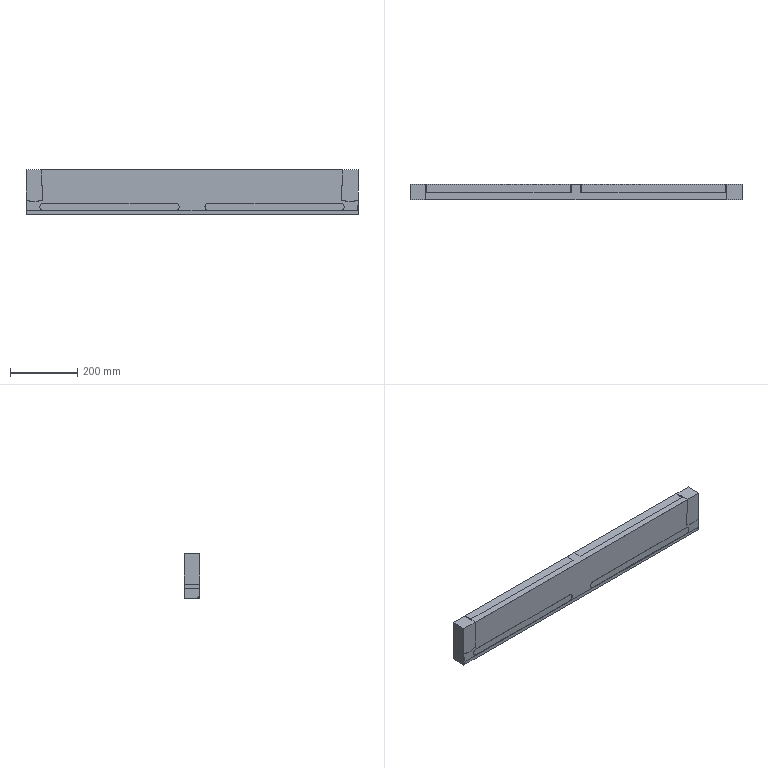NC program | NX | posted with a generic post | part box 987 x 45 x 132.5 mm
Whole program:
N10 G17 G21 G94 G90
(ZLEVEL_PROFILE_COPY_2 , TOOL : D63)
N12 T01 M6
N14 G54
N16 G17 G0 G90 X542.392 Y-19.114 B0. C0. S6500 M3
N18 G43 Z30. H1
N20 Z5.625
N22 G94 G1 X537.561 Y-10.747 F2000.
N24 G3 X532.106 Y-7.597 R6.3
N26 G1 X500.977
N28 X498.032 Y-7.6
N30 X-491.979
N32 X-532.106 Y-7.597
N34 G3 X-537.562 Y-10.746 R6.3
N36 G1 X-542.393 Y-19.113
N38 G0 Z3.75
N40 G1 X-537.562 Y-10.746
N42 G2 X-532.106 Y-7.597 R6.3
N44 G1 X-491.979 Y-7.6
N46 X498.032
N48 X500.977 Y-7.597
N50 X532.106
N52 G2 X537.561 Y-10.747 R6.3
N54 G1 X542.392 Y-19.114
N56 G0 Z1.875
N58 G1 X537.561 Y-10.747
N60 G3 X532.106 Y-7.597 R6.3
N62 G1 X500.977
N64 X498.032 Y-7.6
N66 X-491.979
N68 X-532.106 Y-7.597
N70 G3 X-537.562 Y-10.747 R6.3
N72 G1 X-542.393 Y-19.113
N74 G0 Z0.
N76 G1 X-537.562 Y-10.747
N78 G2 X-532.106 Y-7.597 R6.3
N80 G1 X-491.979 Y-7.6
N82 X498.032
N84 X500.977 Y-7.597
N86 X532.106
N88 G2 X537.561 Y-10.747 R6.3
N90 G1 X542.392 Y-19.114
N92 G0 Z30.
(ZLEVEL_PROFILE , TOOL : D63)
N94 X489.437 Y67.209
N96 Z-1.968
N98 G1 X481.147 Y62.423
N100 G3 X477.997 Y56.967 R6.3
N102 G1 Y24.501
N104 X478. Y22.551
N106 Y-16.867
N108 X477.997 Y-56.967
N110 G3 X481.147 Y-62.423 R6.3
N112 G1 X489.437 Y-67.211
N114 G0 Z-3.936
N116 G1 X481.147 Y-62.423
N118 G2 X477.997 Y-56.967 R6.3
N120 G1 X478. Y-16.867
N122 Y22.551
N124 X477.997 Y24.501
N126 Y56.967
N128 G2 X481.147 Y62.423 R6.3
N130 G1 X489.437 Y67.209
N132 G0 X489.438 Z-5.904
N134 G1 X481.147 Y62.423
N136 G3 X477.997 Y56.967 R6.3
N138 G1 Y24.501
N140 X478. Y22.551
N142 Y-16.867
N144 X477.997 Y-56.967
N146 G3 X481.147 Y-62.423 R6.3
N148 G1 X489.437 Y-67.21
N150 G0 Z-7.872
N152 G1 X481.147 Y-62.423
N154 G2 X477.997 Y-56.967 R6.3
N156 G1 X478. Y-16.867
N158 Y22.551
N160 X477.997 Y24.501
N162 Y56.967
N164 G2 X481.147 Y62.423 R6.3
N166 G1 X489.438 Y67.209
N168 G0 Z-9.84
N170 G1 X481.147 Y62.423
N172 G3 X477.997 Y56.967 R6.3
N174 G1 Y24.501
N176 X478. Y22.551
N178 Y-16.867
N180 X477.997 Y-56.967
N182 G3 X481.147 Y-62.423 R6.3
N184 G1 X489.437 Y-67.21
N186 G0 X489.438 Z-11.809
N188 G1 X481.147 Y-62.423
N190 G2 X477.997 Y-56.967 R6.3
N192 G1 X478. Y-16.867
N194 Y22.551
N196 X477.997 Y24.501
N198 Y56.967
N200 G2 X481.147 Y62.423 R6.3
N202 G1 X489.438 Y67.209
N204 G0 Y67.21 Z-13.777
N206 G1 X481.147 Y62.423
N208 G3 X477.997 Y56.967 R6.3
N210 G1 Y24.501
N212 X478. Y22.551
N214 Y-16.867
N216 X477.997 Y-56.967
N218 G3 X481.147 Y-62.423 R6.3
N220 G1 X489.44 Y-67.212
N222 G0 Y-67.211 Z-15.745
N224 G1 X481.147 Y-62.423
N226 G2 X477.998 Y-56.967 R6.3
N228 G1 X478. Y-16.867
N230 Y22.551
N232 X477.998 Y24.501
N234 Y56.967
N236 G2 X481.148 Y62.423 R6.3
N238 G1 X489.438 Y67.21
N240 G0 Z-17.713
N242 G1 X481.148 Y62.423
N244 G3 X477.998 Y56.967 R6.3
N246 G1 Y24.501
N248 X478. Y22.551
N250 Y-16.867
N252 X477.998 Y-56.967
N254 G3 X481.147 Y-62.423 R6.3
N256 G1 X489.438 Y-67.21
N258 G0 Z-19.681
N260 G1 X481.147 Y-62.423
N262 G2 X477.998 Y-56.967 R6.3
N264 G1 X478. Y-16.867
N266 Y22.551
N268 X477.998 Y24.501
N270 Y56.967
N272 G2 X481.148 Y62.423 R6.3
N274 G1 X489.438 Y67.21
N276 G0 Z-21.649
N278 G1 X481.148 Y62.423
N280 G3 X477.998 Y56.967 R6.3
N282 G1 Y24.501
N284 X478. Y22.551
N286 Y-16.867
N288 X477.998 Y-56.967
N290 G3 X481.147 Y-62.423 R6.3
N292 G1 X489.438 Y-67.21
N294 G0 Z-23.617
N296 G1 X481.148 Y-62.423
N298 G2 X477.998 Y-56.967 R6.3
N300 G1 X478. Y-16.867
N302 Y22.551
N304 X477.998 Y24.501
N306 Y56.967
N308 G2 X481.148 Y62.423 R6.3
N310 G1 X489.438 Y67.21
N312 G0 Z-25.585
N314 G1 X481.148 Y62.423
N316 G3 X477.998 Y56.967 R6.3
N318 G1 Y24.501
N320 X478. Y22.551
N322 Y-16.867
N324 X477.998 Y-56.967
N326 G3 X481.148 Y-62.423 R6.3
N328 G1 X489.438 Y-67.21
N330 G0 Z-27.553
N332 G1 X481.148 Y-62.423
N334 G2 X477.998 Y-56.967 R6.3
N336 G1 X478. Y-16.867
N338 Y22.551
N340 X477.998 Y24.501
N342 Y56.967
N344 G2 X481.148 Y62.423 R6.3
N346 G1 X489.438 Y67.21
N348 G0 Z-29.521
N350 G1 X481.148 Y62.423
N352 G3 X477.998 Y56.967 R6.3
N354 G1 X478. Y22.551
N356 Y-16.867
N358 X477.998 Y-56.967
N360 G3 X481.148 Y-62.423 R6.3
N362 G1 X489.438 Y-67.21
N364 G0 Z-31.489
N366 G1 X481.148 Y-62.423
N368 G2 X477.998 Y-56.967 R6.3
N370 G1 X478. Y-16.867
N372 Y22.551
N374 X477.998 Y56.967
N376 G2 X481.148 Y62.423 R6.3
N378 G1 X489.438 Y67.21
N380 G0 X489.44 Y67.211 Z-33.457
N382 G1 X481.148 Y62.423
N384 G3 X477.998 Y56.967 R6.3
N386 G1 X478. Y22.551
N388 Y-16.867
N390 X477.998 Y-56.967
N392 G3 X481.148 Y-62.423 R6.3
N394 G1 X489.44 Y-67.211
N396 G0 Z-35.426
N398 G1 X481.148 Y-62.423
N400 G2 X477.998 Y-56.967 R6.3
N402 G1 X478. Y-16.867
N404 Y22.551
N406 X477.998 Y56.967
N408 G2 X481.148 Y62.423 R6.3
N410 G1 X489.44 Y67.211
N412 G0 X489.441 Z-37.394
N414 G1 X481.148 Y62.423
N416 G3 X477.998 Y56.967 R6.3
N418 G1 X478. Y22.551
N420 Y-16.867
N422 X477.998 Y-56.967
N424 G3 X481.148 Y-62.423 R6.3
N426 G1 X489.441 Y-67.211
N428 G0 Z-39.362
N430 G1 X481.148 Y-62.423
N432 G2 X477.998 Y-56.967 R6.3
N434 G1 X478. Y-16.867
N436 Y22.551
N438 X477.998 Y56.967
N440 G2 X481.148 Y62.423 R6.3
N442 G1 X489.441 Y67.211
N444 G0 Z-41.33
N446 G1 X481.148 Y62.423
N448 G3 X477.998 Y56.967 R6.3
N450 G1 X478. Y22.551
N452 Y-16.867
N454 X477.998 Y-56.967
N456 G3 X481.148 Y-62.423 R6.3
N458 G1 X489.441 Y-67.211
N460 G0 Z-43.298
N462 G1 X481.148 Y-62.423
N464 G2 X477.999 Y-56.967 R6.3
N466 G1 X478. Y-16.867
N468 Y22.551
N470 X477.999 Y56.967
N472 G2 X481.148 Y62.423 R6.3
N474 G1 X489.441 Y67.211
N476 G0 Z-45.266
N478 G1 X481.148 Y62.423
N480 G3 X477.999 Y56.967 R6.3
N482 G1 X478. Y22.551
N484 Y-16.867
N486 X477.999 Y-56.967
N488 G3 X481.148 Y-62.423 R6.3
N490 G1 X489.441 Y-67.211
N492 G0 Z-47.234
N494 G1 X481.149 Y-62.423
N496 G2 X477.999 Y-56.967 R6.3
N498 G1 X478. Y-16.867
N500 Y22.551
N502 X477.999 Y56.967
N504 G2 X481.148 Y62.423 R6.3
N506 G1 X489.441 Y67.211
N508 G0 Z-49.202
N510 G1 X481.149 Y62.423
N512 G3 X477.999 Y56.967 R6.3
N514 G1 X478. Y22.551
N516 Y-16.867
N518 X477.999 Y-56.967
N520 G3 X481.149 Y-62.423 R6.3
N522 G1 X489.441 Y-67.211
N524 G0 Z-51.17
N526 G1 X481.149 Y-62.423
N528 G2 X477.999 Y-56.967 R6.3
N530 G1 X478. Y-16.867
N532 Y22.551
N534 X477.999 Y56.967
N536 G2 X481.149 Y62.423 R6.3
N538 G1 X489.441 Y67.211
N540 G0 Z-53.138
N542 G1 X481.149 Y62.423
N544 G3 X477.999 Y56.967 R6.3
N546 G1 X478. Y22.551
N548 Y-16.867
N550 X477.999 Y-56.967
N552 G3 X481.149 Y-62.423 R6.3
N554 G1 X489.441 Y-67.211
N556 G0 Z-55.106
N558 G1 X481.149 Y-62.423
N560 G2 X477.999 Y-56.967 R6.3
N562 G1 X478. Y-16.867
N564 Y22.551
N566 X477.999 Y56.967
N568 G2 X481.149 Y62.423 R6.3
N570 G1 X489.441 Y67.211
N572 G0 Z-57.074
N574 G1 X481.149 Y62.423
N576 G3 X477.999 Y56.967 R6.3
N578 G1 X478. Y22.551
N580 Y-16.867
N582 X477.999 Y-56.967
N584 G3 X481.149 Y-62.423 R6.3
N586 G1 X489.441 Y-67.211
N588 G0 Z-59.043
N590 G1 X481.149 Y-62.423
N592 G2 X477.999 Y-56.967 R6.3
N594 G1 X478. Y-16.867
N596 Y22.551
N598 X477.999 Y56.967
N600 G2 X481.149 Y62.423 R6.3
N602 G1 X489.441 Y67.211
N604 G0 Z-61.011
N606 G1 X481.149 Y62.423
N608 G3 X477.999 Y56.967 R6.3
N610 G1 X478. Y22.551
N612 Y-16.867
N614 X477.999 Y-56.967
N616 G3 X481.149 Y-62.423 R6.3
N618 G1 X489.441 Y-67.211
N620 G0 Z-62.979
N622 G1 X481.149 Y-62.423
N624 G2 X477.999 Y-56.967 R6.3
N626 G1 X478. Y-16.867
N628 Y22.551
N630 X477.999 Y56.967
N632 G2 X481.149 Y62.423 R6.3
N634 G1 X489.441 Y67.211
N636 G0 X489.442 Z-64.947
N638 G1 X481.149 Y62.423
N640 G3 X477.999 Y56.967 R6.3
N642 G1 X478. Y22.551
N644 Y-16.867
N646 X477.999 Y-56.967
N648 G3 X481.149 Y-62.423 R6.3
N650 G1 X489.442 Y-67.211
N652 G0 Z-66.915
N654 G1 X481.149 Y-62.423
N656 G2 X477.999 Y-56.967 R6.3
N658 G1 X478. Y-16.867
N660 Y22.551
N662 X477.999 Y56.967
N664 G2 X481.149 Y62.423 R6.3
N666 G1 X489.442 Y67.211
N668 G0 Z-68.883
N670 G1 X481.149 Y62.423
N672 G3 X477.999 Y56.967 R6.3
N674 G1 X478. Y22.551
N676 Y-16.867
N678 X477.999 Y-56.967
N680 G3 X481.149 Y-62.423 R6.3
N682 G1 X489.442 Y-67.211
N684 G0 Z-70.851
N686 G1 X481.15 Y-62.423
N688 G2 X478. Y-56.967 R6.3
N690 G1 Y-16.867
N692 Y22.551
N694 Y56.967
N696 G2 X481.149 Y62.423 R6.3
N698 G1 X489.442 Y67.211
N700 G0 Z-72.819
N702 G1 X481.15 Y62.423
N704 G3 X478. Y56.967 R6.3
N706 G1 Y22.551
N708 Y-16.867
N710 Y-56.967
N712 G3 X481.15 Y-62.423 R6.3
N714 G1 X489.442 Y-67.211
N716 G0 Z-74.787
N718 G1 X481.15 Y-62.423
N720 G2 X478. Y-56.967 R6.3
N722 G1 Y-16.867
N724 Y22.551
N726 Y56.967
N728 G2 X481.15 Y62.423 R6.3
N730 G1 X489.442 Y67.211
N732 G0 Z-76.755
N734 G1 X481.15 Y62.423
N736 G3 X478. Y56.967 R6.3
N738 G1 Y22.551
N740 Y-16.867
N742 Y-56.967
N744 G3 X481.15 Y-62.423 R6.3
N746 G1 X489.442 Y-67.211
N748 G0 Z-78.723
N750 G1 X481.15 Y-62.423
N752 G2 X478. Y-56.967 R6.3
N754 G1 Y-16.867
N756 Y22.551
N758 Y56.967
N760 G2 X481.15 Y62.423 R6.3
N762 G1 X489.442 Y67.211
N764 G0 Z-80.691
N766 G1 X481.15 Y62.423
N768 G3 X478. Y56.967 R6.3
N770 G1 Y22.551
N772 Y-16.867
N774 Y-56.967
N776 G3 X481.15 Y-62.423 R6.3
N778 G1 X489.442 Y-67.211
N780 G0 Z-82.66
N782 G1 X481.15 Y-62.423
N784 G2 X478. Y-56.967 R6.3
N786 G1 Y-16.867
N788 Y22.463
N790 Y56.967
N792 G2 X481.15 Y62.423 R6.3
N794 G1 X489.442 Y67.211
N796 G0 Z-84.628
N798 G1 X481.15 Y62.423
N800 G3 X478. Y56.967 R6.3
N802 G1 Y22.463
N804 Y-16.867
N806 Y-56.967
N808 G3 X481.15 Y-62.423 R6.3
N810 G1 X489.442 Y-67.211
N812 G0 Z-86.596
N814 G1 X481.15 Y-62.423
N816 G2 X478. Y-56.967 R6.3
N818 G1 Y-16.867
N820 Y22.463
N822 Y56.967
N824 G2 X481.15 Y62.423 R6.3
N826 G1 X489.442 Y67.211
N828 G0 Z-88.564
N830 G1 X481.15 Y62.423
N832 G3 X478. Y56.967 R6.3
N834 G1 Y22.463
N836 Y-16.867
N838 Y-56.967
N840 G3 X481.15 Y-62.423 R6.3
N842 G1 X489.442 Y-67.211
N844 G0 Z-90.532
N846 G1 X481.15 Y-62.423
N848 G2 X478. Y-56.967 R6.3
N850 G1 Y-16.867
N852 Y22.463
N854 Y56.967
N856 G2 X481.15 Y62.423 R6.3
N858 G1 X489.442 Y67.211
N860 G0 Z-92.5
N862 G1 X481.15 Y62.423
N864 G3 X478. Y56.967 R6.3
N866 G1 Y22.463
N868 Y-16.867
N870 Y-56.967
N872 G3 X481.15 Y-62.423 R6.3
N874 G1 X489.442 Y-67.211
N876 G0 Z30.
N878 X-489.437
N880 Z-1.968
N882 G1 X-481.147 Y-62.423
N884 G3 X-477.997 Y-56.967 R6.3
N886 G1 X-478. Y-16.897
N888 Y22.5
N890 X-477.997 Y56.967
N892 G3 X-481.147 Y62.423 R6.3
N894 G1 X-489.437 Y67.211
N896 G0 X-489.435 Y67.218 Z-3.936
N898 G1 X-481.144 Y62.425
N900 G2 X-477.997 Y56.967 R6.3
N902 G1 X-477.999 Y53.105
N904 X-478. Y22.5
N906 Y-16.897
N908 X-477.997 Y-56.967
N910 G2 X-481.147 Y-62.423 R6.3
N912 G1 X-489.437 Y-67.211
N914 G0 Y-67.21 Z-5.904
N916 G1 X-481.147 Y-62.423
N918 G3 X-477.997 Y-56.967 R6.3
N920 G1 X-478. Y-16.897
N922 Y22.5
N924 X-477.999 Y53.105
N926 X-477.997 Y56.967
N928 G3 X-481.144 Y62.425 R6.3
N930 G1 X-489.436 Y67.218
N932 G0 X-489.437 Y67.211 Z-7.872
N934 G1 X-481.147 Y62.423
N936 G2 X-477.997 Y56.967 R6.3
N938 G1 X-478. Y22.5
N940 Y-16.897
N942 X-477.997 Y-56.967
N944 G2 X-481.147 Y-62.423 R6.3
N946 G1 X-489.437 Y-67.21
N948 G0 Z-9.84
N950 G1 X-481.147 Y-62.423
N952 G3 X-477.997 Y-56.967 R6.3
N954 G1 X-478. Y-16.897
N956 Y22.5
N958 X-477.997 Y56.967
N960 G3 X-481.147 Y62.423 R6.3
N962 G1 X-489.437 Y67.211
N964 G0 Z-11.809
N966 G1 X-481.147 Y62.423
N968 G2 X-477.997 Y56.967 R6.3
N970 G1 X-478. Y22.5
N972 Y-16.897
N974 X-477.997 Y-56.967
N976 G2 X-481.147 Y-62.423 R6.3
N978 G1 X-489.438 Y-67.21
N980 G0 Y-67.211 Z-13.777
N982 G1 X-481.147 Y-62.423
N984 G3 X-477.997 Y-56.967 R6.3
N986 G1 X-478. Y-16.897
N988 Y22.5
N990 X-477.997 Y56.967
N992 G3 X-481.147 Y62.423 R6.3
N994 G1 X-489.44 Y67.212
N996 G0 Z-15.745
N998 G1 X-481.147 Y62.423
N1000 G2 X-477.998 Y56.967 R6.3
N1002 G1 X-478. Y22.5
N1004 Y-16.897
N1006 X-477.998 Y-56.967
N1008 G2 X-481.147 Y-62.423 R6.3
N1010 G1 X-489.438 Y-67.21
N1012 G0 Z-17.713
N1014 G1 X-481.147 Y-62.423
N1016 G3 X-477.998 Y-56.967 R6.3
N1018 G1 X-478. Y-16.897
N1020 Y22.5
N1022 X-477.998 Y56.967
N1024 G3 X-481.147 Y62.423 R6.3
N1026 G1 X-489.438 Y67.211
N1028 G0 Z-19.681
N1030 G1 X-481.147 Y62.423
N1032 G2 X-477.998 Y56.967 R6.3
N1034 G1 X-478. Y22.5
N1036 Y-16.897
N1038 X-477.998 Y-56.967
N1040 G2 X-481.147 Y-62.423 R6.3
N1042 G1 X-489.438 Y-67.21
N1044 G0 Z-21.649
N1046 G1 X-481.147 Y-62.423
N1048 G3 X-477.998 Y-56.967 R6.3
N1050 G1 X-478. Y-16.897
N1052 Y22.5
N1054 X-477.998 Y56.967
N1056 G3 X-481.147 Y62.423 R6.3
N1058 G1 X-489.438 Y67.211
N1060 G0 Y67.21 Z-23.617
N1062 G1 X-481.147 Y62.423
N1064 G2 X-477.998 Y56.967 R6.3
N1066 G1 X-478. Y22.5
N1068 Y-16.897
N1070 X-477.998 Y-56.967
N1072 G2 X-481.148 Y-62.423 R6.3
N1074 G1 X-489.438 Y-67.21
N1076 G0 Z-25.585
N1078 G1 X-481.148 Y-62.423
N1080 G3 X-477.998 Y-56.967 R6.3
N1082 G1 X-478. Y-16.897
N1084 Y22.5
N1086 X-477.998 Y56.967
N1088 G3 X-481.148 Y62.423 R6.3
N1090 G1 X-489.438 Y67.21
N1092 G0 Z-27.553
N1094 G1 X-481.148 Y62.423
N1096 G2 X-477.998 Y56.967 R6.3
N1098 G1 X-478. Y22.5
N1100 Y-16.897
N1102 X-477.998 Y-56.967
N1104 G2 X-481.148 Y-62.423 R6.3
N1106 G1 X-489.438 Y-67.21
N1108 G0 Z-29.521
N1110 G1 X-481.148 Y-62.423
N1112 G3 X-477.998 Y-56.967 R6.3
N1114 G1 X-478. Y-16.897
N1116 Y22.5
N1118 X-477.998 Y56.967
N1120 G3 X-481.148 Y62.423 R6.3
N1122 G1 X-489.438 Y67.21
N1124 G0 Z-31.489
N1126 G1 X-481.148 Y62.423
N1128 G2 X-477.998 Y56.967 R6.3
N1130 G1 X-478. Y22.5
N1132 Y-16.897
N1134 X-477.998 Y-56.967
N1136 G2 X-481.148 Y-62.423 R6.3
N1138 G1 X-489.438 Y-67.21
N1140 G0 X-489.44 Y-67.211 Z-33.457
N1142 G1 X-481.148 Y-62.423
N1144 G3 X-477.998 Y-56.967 R6.3
N1146 G1 X-478. Y-16.897
N1148 Y22.5
N1150 X-477.998 Y56.967
N1152 G3 X-481.148 Y62.423 R6.3
N1154 G1 X-489.44 Y67.211
N1156 G0 Z-35.426
N1158 G1 X-481.148 Y62.423
N1160 G2 X-477.998 Y56.967 R6.3
N1162 G1 X-478. Y22.5
N1164 Y-16.897
N1166 X-477.998 Y-56.967
N1168 G2 X-481.148 Y-62.423 R6.3
N1170 G1 X-489.44 Y-67.211
N1172 G0 X-489.441 Z-37.394
N1174 G1 X-481.148 Y-62.423
N1176 G3 X-477.998 Y-56.967 R6.3
N1178 G1 X-478. Y-16.897
N1180 Y22.5
N1182 X-477.998 Y56.967
N1184 G3 X-481.148 Y62.423 R6.3
N1186 G1 X-489.441 Y67.211
N1188 G0 Z-39.362
N1190 G1 X-481.148 Y62.423
N1192 G2 X-477.998 Y56.967 R6.3
N1194 G1 X-478. Y22.5
N1196 Y-16.897
N1198 X-477.998 Y-56.967
N1200 G2 X-481.148 Y-62.423 R6.3
N1202 G1 X-489.441 Y-67.211
N1204 G0 Z-41.33
N1206 G1 X-481.148 Y-62.423
N1208 G3 X-477.998 Y-56.967 R6.3
N1210 G1 X-478. Y-16.897
N1212 Y22.5
N1214 X-477.998 Y56.967
N1216 G3 X-481.148 Y62.423 R6.3
N1218 G1 X-489.441 Y67.211
N1220 G0 Z-43.298
N1222 G1 X-481.148 Y62.423
N1224 G2 X-477.999 Y56.967 R6.3
N1226 G1 X-478. Y22.5
N1228 Y-16.897
N1230 X-477.999 Y-56.967
N1232 G2 X-481.148 Y-62.423 R6.3
N1234 G1 X-489.441 Y-67.211
N1236 G0 Z-45.266
N1238 G1 X-481.148 Y-62.423
N1240 G3 X-477.999 Y-56.967 R6.3
N1242 G1 X-478. Y-16.897
N1244 Y22.5
N1246 X-477.999 Y56.967
N1248 G3 X-481.148 Y62.423 R6.3
N1250 G1 X-489.441 Y67.211
N1252 G0 Z-47.234
N1254 G1 X-481.148 Y62.423
N1256 G2 X-477.999 Y56.967 R6.3
N1258 G1 X-478. Y22.5
N1260 Y-16.897
N1262 X-477.999 Y-56.967
N1264 G2 X-481.149 Y-62.423 R6.3
N1266 G1 X-489.441 Y-67.211
N1268 G0 Z-49.202
N1270 G1 X-481.149 Y-62.423
N1272 G3 X-477.999 Y-56.967 R6.3
N1274 G1 X-478. Y-16.867
N1276 Y22.5
N1278 X-477.999 Y56.967
N1280 G3 X-481.149 Y62.423 R6.3
N1282 G1 X-489.441 Y67.211
N1284 G0 Z-51.17
N1286 G1 X-481.149 Y62.423
N1288 G2 X-477.999 Y56.967 R6.3
N1290 G1 X-478. Y22.5
N1292 Y-16.867
N1294 X-477.999 Y-56.967
N1296 G2 X-481.149 Y-62.423 R6.3
N1298 G1 X-489.441 Y-67.211
N1300 G0 Z-53.138
N1302 G1 X-481.149 Y-62.423
N1304 G3 X-477.999 Y-56.967 R6.3
N1306 G1 X-478. Y-16.867
N1308 Y22.5
N1310 X-477.999 Y56.967
N1312 G3 X-481.149 Y62.423 R6.3
N1314 G1 X-489.441 Y67.211
N1316 G0 Z-55.106
N1318 G1 X-481.149 Y62.423
N1320 G2 X-477.999 Y56.967 R6.3
N1322 G1 X-478. Y22.5
N1324 Y-16.867
N1326 X-477.999 Y-56.967
N1328 G2 X-481.149 Y-62.423 R6.3
N1330 G1 X-489.441 Y-67.211
N1332 G0 Z-57.074
N1334 G1 X-481.149 Y-62.423
N1336 G3 X-477.999 Y-56.967 R6.3
N1338 G1 X-478. Y-16.867
N1340 Y22.5
N1342 X-477.999 Y56.967
N1344 G3 X-481.149 Y62.423 R6.3
N1346 G1 X-489.441 Y67.211
N1348 G0 Z-59.043
N1350 G1 X-481.149 Y62.423
N1352 G2 X-477.999 Y56.967 R6.3
N1354 G1 X-478. Y22.5
N1356 Y-16.867
N1358 X-477.999 Y-56.967
N1360 G2 X-481.149 Y-62.423 R6.3
N1362 G1 X-489.441 Y-67.211
N1364 G0 Z-61.011
N1366 G1 X-481.149 Y-62.423
N1368 G3 X-477.999 Y-56.967 R6.3
N1370 G1 X-478. Y-16.867
N1372 Y22.5
N1374 X-477.999 Y56.967
N1376 G3 X-481.149 Y62.423 R6.3
N1378 G1 X-489.441 Y67.211
N1380 G0 Z-62.979
N1382 G1 X-481.149 Y62.423
N1384 G2 X-477.999 Y56.967 R6.3
N1386 G1 X-478. Y22.5
N1388 Y-16.867
N1390 X-477.999 Y-56.967
N1392 G2 X-481.149 Y-62.423 R6.3
N1394 G1 X-489.441 Y-67.211
N1396 G0 X-489.442 Z-64.947
N1398 G1 X-481.149 Y-62.423
N1400 G3 X-477.999 Y-56.967 R6.3
N1402 G1 X-478. Y-16.867
N1404 Y22.5
N1406 X-477.999 Y56.967
N1408 G3 X-481.149 Y62.423 R6.3
N1410 G1 X-489.442 Y67.211
N1412 G0 Z-66.915
N1414 G1 X-481.149 Y62.423
N1416 G2 X-477.999 Y56.967 R6.3
N1418 G1 X-478. Y22.5
N1420 Y-16.867
N1422 X-477.999 Y-56.967
N1424 G2 X-481.149 Y-62.423 R6.3
N1426 G1 X-489.442 Y-67.211
N1428 G0 Z-68.883
N1430 G1 X-481.149 Y-62.423
N1432 G3 X-477.999 Y-56.967 R6.3
N1434 G1 X-478. Y-16.867
N1436 Y22.5
N1438 X-477.999 Y56.967
N1440 G3 X-481.149 Y62.423 R6.3
N1442 G1 X-489.442 Y67.211
N1444 G0 Z-70.851
N1446 G1 X-481.149 Y62.423
N1448 G2 X-478. Y56.967 R6.3
N1450 G1 Y22.5
N1452 Y-16.867
N1454 Y-56.967
N1456 G2 X-481.15 Y-62.423 R6.3
N1458 G1 X-489.442 Y-67.211
N1460 G0 Z-72.819
N1462 G1 X-481.15 Y-62.423
N1464 G3 X-478. Y-56.967 R6.3
N1466 G1 Y-16.867
N1468 Y22.5
N1470 Y56.967
N1472 G3 X-481.15 Y62.423 R6.3
N1474 G1 X-489.442 Y67.211
N1476 G0 Z-74.787
N1478 G1 X-481.15 Y62.423
N1480 G2 X-478. Y56.967 R6.3
N1482 G1 Y22.5
N1484 Y-16.867
N1486 Y-56.967
N1488 G2 X-481.15 Y-62.423 R6.3
N1490 G1 X-489.442 Y-67.211
N1492 G0 Z-76.755
N1494 G1 X-481.15 Y-62.423
N1496 G3 X-478. Y-56.967 R6.3
N1498 G1 Y-16.867
N1500 Y22.5
N1502 Y56.967
N1504 G3 X-481.15 Y62.423 R6.3
N1506 G1 X-489.442 Y67.211
N1508 G0 Z-78.723
N1510 G1 X-481.15 Y62.423
N1512 G2 X-478. Y56.967 R6.3
N1514 G1 Y22.5
N1516 Y-16.867
N1518 Y-56.967
N1520 G2 X-481.15 Y-62.423 R6.3
N1522 G1 X-489.442 Y-67.211
N1524 G0 Z-80.691
N1526 G1 X-481.15 Y-62.423
N1528 G3 X-478. Y-56.967 R6.3
N1530 G1 Y-16.867
N1532 Y22.5
N1534 Y56.967
N1536 G3 X-481.15 Y62.423 R6.3
N1538 G1 X-489.442 Y67.211
N1540 G0 Z-82.66
N1542 G1 X-481.15 Y62.423
N1544 G2 X-478. Y56.967 R6.3
N1546 G1 Y23.897
N1548 X-477.97 Y23.866
N1550 G3 X-478. Y22.5 R31.6
N1552 G1 Y-16.867
N1554 Y-56.967
N1556 G2 X-481.15 Y-62.423 R6.3
N1558 G1 X-489.442 Y-67.211
N1560 G0 Z-84.628
N1562 G1 X-481.15 Y-62.423
N1564 G3 X-478. Y-56.967 R6.3
N1566 G1 Y-16.867
N1568 Y22.5
N1570 G2 X-477.97 Y23.866 R31.6
N1572 G1 X-478.001 Y23.897
N1574 X-478. Y56.967
N1576 G3 X-481.15 Y62.423 R6.3
N1578 G1 X-489.442 Y67.211
N1580 G0 Z-86.596
N1582 G1 X-481.15 Y62.423
N1584 G2 X-478. Y56.967 R6.3
N1586 G1 X-478.002 Y23.897
N1588 X-477.97 Y23.866
N1590 G3 X-478. Y22.5 R31.6
N1592 G1 Y-16.867
N1594 Y-56.967
N1596 G2 X-481.15 Y-62.423 R6.3
N1598 G1 X-489.442 Y-67.211
N1600 G0 Z-88.564
N1602 G1 X-481.15 Y-62.423
N1604 G3 X-478. Y-56.967 R6.3
N1606 G1 Y-16.867
N1608 Y22.5
N1610 G2 X-477.97 Y23.866 R31.6
N1612 G1 X-478.002 Y23.897
N1614 Y53.105
N1616 X-478. Y56.967
N1618 G3 X-481.146 Y62.425 R6.3
N1620 G1 X-489.44 Y67.22
N1622 G0 X-489.439 Y67.223 Z-90.532
N1624 G1 X-481.145 Y62.426
N1626 G2 X-478. Y56.967 R6.3
N1628 G1 X-478.003 Y53.105
N1630 Y23.897
N1632 X-477.97 Y23.866
N1634 G3 X-478. Y22.5 R31.6
N1636 G1 Y-16.867
N1638 Y-56.967
N1640 G2 X-481.15 Y-62.423 R6.3
N1642 G1 X-489.442 Y-67.211
N1644 G0 Z-92.5
N1646 G1 X-481.15 Y-62.423
N1648 G3 X-478. Y-56.967 R6.3
N1650 G1 Y-16.867
N1652 Y22.5
N1654 G2 X-477.97 Y23.866 R31.6
N1656 G1 X-478.004 Y23.897
N1658 X-478. Y56.967
N1660 G3 X-481.149 Y62.423 R6.3
N1662 G1 X-489.442 Y67.212
N1664 G0 Z30.
N1666 M5
(CUTTERCOMP9 , TOOL : D16)
N1668 T16 M6
N1670 G54
N1672 G17 G0 G90 X457.615 Y32.646 B0. C0. S6500 M3
N1674 G43 Z30. H16
N1676 Z-14.783
N1678 G94 G1 Z-15.783 F1000.
N1680 G41 X457.515 D16
N1682 X455.72 Y32.329
N1684 G3 X454.398 Y30.753 R1.6
N1686 G1 X454.4 Y22.5
N1688 Y-20.561
N1690 X454.398 Y-30.753
N1692 G3 X455.72 Y-32.329 R1.6
N1694 G1 X457.517 Y-32.646
N1696 G40
N1698 X457.617
N1700 Z-14.783
N1702 G0 X457.615 Y32.645 Z-30.567
N1704 G1 Z-31.567
N1706 G41 X457.515
N1708 X455.721 Y32.329
N1710 G3 X454.399 Y30.753 R1.6
N1712 G1 X454.4 Y22.5
N1714 Y-20.561
N1716 X454.399 Y-30.753
N1718 G3 X455.721 Y-32.329 R1.6
N1720 G1 X457.518 Y-32.646
N1722 G40
N1724 X457.618
N1726 Z-30.567
N1728 G0 X457.616 Y32.645 Z-46.35
N1730 G1 Z-47.35
N1732 G41 X457.516
N1734 X455.722 Y32.329
N1736 G3 X454.4 Y30.753 R1.6
N1738 G1 Y22.5
N1740 Y-20.561
N1742 Y-30.753
N1744 G3 X455.722 Y-32.329 R1.6
N1746 G1 X457.518 Y-32.646
N1748 G40
N1750 X457.618
N1752 Z-46.35
N1754 G0 Z30.
N1756 X-457.616
N1758 Z-14.783
N1760 G1 Z-15.783
N1762 G41 X-457.516
N1764 X-455.719 Y-32.329
N1766 G3 X-454.398 Y-30.753 R1.6
N1768 G1 X-454.4 Y-20.561
N1770 Y22.5
N1772 X-454.398 Y30.753
N1774 G3 X-455.719 Y32.329 R1.6
N1776 G1 X-457.516 Y32.646
N1778 G40
N1780 X-457.616
N1782 Z-14.783
N1784 G0 X-457.617 Y-32.646 Z-30.567
N1786 G1 Z-31.567
N1788 G41 X-457.517
N1790 X-455.72 Y-32.329
N1792 G3 X-454.398 Y-30.753 R1.6
N1794 G1 X-454.4 Y-20.561
N1796 Y22.5
N1798 X-454.398 Y30.753
N1800 G3 X-455.72 Y32.329 R1.6
N1802 G1 X-457.517 Y32.646
N1804 G40
N1806 X-457.617
N1808 Z-30.567
N1810 G0 Y-32.646 Z-46.35
N1812 G1 Z-47.35
N1814 G41 X-457.517
N1816 X-455.72 Y-32.329
N1818 G3 X-454.398 Y-30.753 R1.6
N1820 G1 X-454.4 Y-20.561
N1822 Y22.5
N1824 X-454.398 Y30.753
N1826 G3 X-455.72 Y32.329 R1.6
N1828 G1 X-457.517 Y32.646
N1830 G40
N1832 X-457.617
N1834 Z-46.35
N1836 G0 Z30.
(ZLEVEL_PROFILE_COPY , TOOL : D16)
N1838 X468.488 Y33.509
N1840 Z-93.275
N1842 G1 X466.297 Y32.243 F2000.
N1844 G3 X465.497 Y30.857 R1.6
N1846 G1 X465.5 Y22.533
N1848 Y-22.041
N1850 X465.497 Y-30.857
N1852 G3 X466.297 Y-32.243 R1.6
N1854 G1 X468.488 Y-33.509
N1856 G0 Z-94.05
N1858 G1 X466.297 Y-32.243
N1860 G2 X465.497 Y-30.857 R1.6
N1862 G1 X465.5 Y-22.041
N1864 Y22.533
N1866 X465.497 Y30.857
N1868 G2 X466.297 Y32.243 R1.6
N1870 G1 X468.488 Y33.509
N1872 G0 X468.486 Y33.518 Z-94.825
N1874 G1 X466.294 Y32.245
N1876 G3 X465.497 Y30.857 R1.6
N1878 G1 X465.5 Y29.878
N1880 Y22.533
N1882 Y-22.041
N1884 Y-29.878
N1886 X465.497 Y-30.857
N1888 G3 X466.294 Y-32.245 R1.6
N1890 G1 X468.486 Y-33.518
N1892 G0 Y-33.519 Z-95.6
N1894 G1 X466.294 Y-32.245
N1896 G2 X465.498 Y-30.857 R1.6
N1898 G1 X465.5 Y-29.878
N1900 Y-22.041
N1902 Y22.443
N1904 Y29.878
N1906 X465.498 Y30.857
N1908 G2 X466.294 Y32.245 R1.6
N1910 G1 X468.486 Y33.519
N1912 G0 Z30.
N1914 X471.512 Y-33.509
N1916 Z-93.275
N1918 G1 X473.703 Y-32.243
N1920 G3 X474.503 Y-30.857 R1.6
N1922 G1 X474.5 Y-22.041
N1924 Y22.5
N1926 X474.559 Y23.473
N1928 X474.501 Y23.51
N1930 X474.503 Y30.857
N1932 G3 X473.703 Y32.243 R1.6
N1934 G1 X471.512 Y33.509
N1936 G0 Z-94.05
N1938 G1 X473.703 Y32.243
N1940 G2 X474.503 Y30.857 R1.6
N1942 G1 X474.501 Y23.51
N1944 X474.559 Y23.473
N1946 X474.5 Y22.5
N1948 Y-22.041
N1950 X474.503 Y-30.857
N1952 G2 X473.703 Y-32.243 R1.6
N1954 G1 X471.512 Y-33.509
N1956 G0 X471.514 Y-33.518 Z-94.825
N1958 G1 X473.706 Y-32.245
N1960 G3 X474.503 Y-30.857 R1.6
N1962 G1 X474.5 Y-29.878
N1964 Y-22.041
N1966 Y22.5
N1968 X474.559 Y23.473
N1970 X474.5 Y23.51
N1972 Y29.878
N1974 X474.503 Y30.857
N1976 G3 X473.706 Y32.245 R1.6
N1978 G1 X471.514 Y33.518
N1980 G0 Y33.519 Z-95.6
N1982 G1 X473.706 Y32.245
N1984 G2 X474.502 Y30.857 R1.6
N1986 G1 X474.5 Y29.878
N1988 Y23.51
N1990 X474.559 Y23.473
N1992 X474.5 Y22.5
N1994 Y-22.041
N1996 Y-29.878
N1998 X474.502 Y-30.857
N2000 G2 X473.706 Y-32.245 R1.6
N2002 G1 X471.514 Y-33.519
N2004 G0 Z30.
N2006 X-471.512 Y33.509
N2008 Z-93.275
N2010 G1 X-473.703 Y32.243
N2012 G3 X-474.503 Y30.857 R1.6
N2014 G1 X-474.5 Y22.443
N2016 Y-22.041
N2018 X-474.496 Y-23.02
N2020 Y-29.878
N2022 X-474.503 Y-30.857
N2024 G3 X-473.713 Y-32.249 R1.6
N2026 G1 X-471.518 Y-33.537
N2028 G0 Y-33.538 Z-94.05
N2030 G1 X-473.713 Y-32.249
N2032 G2 X-474.503 Y-30.857 R1.6
N2034 G1 X-474.496 Y-29.878
N2036 Y-23.02
N2038 X-474.5 Y-22.041
N2040 Y22.443
N2042 X-474.503 Y30.857
N2044 G2 X-473.703 Y32.243 R1.6
N2046 G1 X-471.512 Y33.509
N2048 G0 Z-94.825
N2050 G1 X-473.703 Y32.243
N2052 G3 X-474.503 Y30.857 R1.6
N2054 G1 X-474.5 Y22.443
N2056 Y-22.041
N2058 X-474.495 Y-23.02
N2060 Y-29.878
N2062 X-474.503 Y-30.857
N2064 G3 X-473.713 Y-32.249 R1.6
N2066 G1 X-471.518 Y-33.539
N2068 G0 Y-33.54 Z-95.6
N2070 G1 X-473.713 Y-32.249
N2072 G2 X-474.502 Y-30.857 R1.6
N2074 G1 X-474.495 Y-29.878
N2076 Y-23.02
N2078 X-474.5 Y-22.041
N2080 Y22.443
N2082 X-474.502 Y30.857
N2084 G2 X-473.703 Y32.243 R1.6
N2086 G1 X-471.512 Y33.509
N2088 G0 Z30.
N2090 X-468.482 Y-33.537
N2092 Z-93.275
N2094 G1 X-466.287 Y-32.249
N2096 G3 X-465.497 Y-30.857 R1.6
N2098 G1 X-465.504 Y-29.878
N2100 Y-23.02
N2102 X-465.5 Y-22.041
N2104 Y22.443
N2106 X-465.504 Y22.5
N2108 X-465.445 Y23.442
N2110 X-465.504 Y23.48
N2112 Y29.878
N2114 X-465.497 Y30.857
N2116 G3 X-466.287 Y32.249 R1.6
N2118 G1 X-468.482 Y33.537
N2120 G0 Y33.538 Z-94.05
N2122 G1 X-466.287 Y32.249
N2124 G2 X-465.497 Y30.857 R1.6
N2126 G1 X-465.504 Y29.878
N2128 Y23.48
N2130 X-465.445 Y23.442
N2132 X-465.504 Y22.5
N2134 X-465.5 Y22.443
N2136 Y-22.041
N2138 X-465.504 Y-23.02
N2140 Y-29.878
N2142 X-465.497 Y-30.857
N2144 G2 X-466.287 Y-32.249 R1.6
N2146 G1 X-468.482 Y-33.538
N2148 G0 Y-33.539 Z-94.825
N2150 G1 X-466.287 Y-32.249
N2152 G3 X-465.497 Y-30.857 R1.6
N2154 G1 X-465.505 Y-29.878
N2156 Y-23.02
N2158 X-465.5 Y-22.041
N2160 Y22.443
N2162 X-465.505 Y22.5
N2164 X-465.445 Y23.442
N2166 X-465.505 Y23.48
N2168 Y29.878
N2170 X-465.497 Y30.857
N2172 G3 X-466.287 Y32.249 R1.6
N2174 G1 X-468.482 Y33.539
N2176 G0 Y33.54 Z-95.6
N2178 G1 X-466.287 Y32.249
N2180 G2 X-465.498 Y30.857 R1.6
N2182 G1 X-465.505 Y29.878
N2184 Y23.449
N2186 X-465.448 Y23.412
N2188 X-465.505 Y22.5
N2190 X-465.5 Y22.443
N2192 Y-22.041
N2194 X-465.505 Y-23.02
N2196 Y-29.878
N2198 X-465.498 Y-30.857
N2200 G2 X-466.287 Y-32.249 R1.6
N2202 G1 X-468.482 Y-33.54
N2204 G0 Z30.
(CUTTERCOMP9_COPY , TOOL : D16)
N2206 X471.383 Y-32.646
N2208 Z-94.6
N2210 G1 Z-95.6 F1000.
N2212 G41 X471.483
N2214 X473.28 Y-32.329
N2216 G3 X474.602 Y-30.753 R1.6
N2218 G1 X474.6 Y-22.289
N2220 X474.599 Y22.5
N2222 X474.619 Y23.046
N2224 X474.599 Y23.065
N2226 Y30.189
N2228 X474.602 Y30.753
N2230 G3 X473.287 Y32.334 R1.6
N2232 G1 X471.485 Y32.66
N2234 G40
N2236 X471.385 Y32.661
N2238 Z-94.6
N2240 G0 Z30.
N2242 X468.614 Y32.656
N2244 Z-94.6
N2246 G1 Z-95.6
N2248 G41 X468.514
N2250 X466.716 Y32.333
N2252 G3 X465.399 Y30.753 R1.6
N2254 G1 X465.401 Y30.189
N2256 X465.4 Y22.487
N2258 Y-22.289
N2260 X465.399 Y-30.753
N2262 G3 X466.721 Y-32.329 R1.6
N2264 G1 X468.516 Y-32.646
N2266 G40
N2268 X468.616
N2270 Z-94.6
N2272 G0 Z30.
N2274 X-468.617
N2276 Z-94.6
N2278 G1 Z-95.6
N2280 G41 X-468.517
N2282 X-466.72 Y-32.329
N2284 G3 X-465.398 Y-30.753 R1.6
N2286 G1 X-465.4 Y-22.289
N2288 Y22.487
N2290 X-465.402 Y22.5
N2292 X-465.383 Y23.028
N2294 X-465.402 Y23.047
N2296 Y30.189
N2298 X-465.398 Y30.753
N2300 G3 X-466.709 Y32.338 R1.6
N2302 G1 X-468.514 Y32.669
N2304 G40
N2306 X-468.614
N2308 Z-94.6
N2310 G0 Z30.
N2312 X-471.387 Y32.665
N2314 Z-94.6
N2316 G1 Z-95.6
N2318 G41 X-471.487 Y32.664
N2320 X-473.288 Y32.336
N2322 G3 X-474.601 Y30.753 R1.6
N2324 G1 X-474.598 Y30.189
N2326 X-474.6 Y22.487
N2328 Y-22.289
N2330 X-474.601 Y-30.753
N2332 G3 X-473.279 Y-32.329 R1.6
N2334 G1 X-471.484 Y-32.646
N2336 G40
N2338 X-471.384
N2340 Z-94.6
N2342 G0 Z30.
N2344 M5
(PLANAR_MILL_1 , TOOL : D10A45)
N2346 T07 M6
N2348 G54
N2350 G17 G0 G90 X1.732 Y-25. B0. C0. S7500 M3
N2352 G43 Z30. H7
N2354 Z2.
N2356 G94 G1 Z-1. F1250.
N2358 X0.866 Y-23.5
N2360 G3 X0. Y-23. R1.
N2362 G1 X-445.9
N2364 G2 X-446.9 Y-22. R1.
N2366 G1 Y22.
N2368 G2 X-445.9 Y23. R1.
N2370 G1 X445.9
N2372 G2 X446.9 Y22. R1.
N2374 G1 Y-22.
N2376 G2 X445.9 Y-23. R1.
N2378 G1 X0.
N2380 G3 X-0.866 Y-23.5 R1.
N2382 G1 X-1.732 Y-25.
N2384 Z2.
N2386 G0 Z30.
N2388 M5
(ZLEVEL_PROFILE_1_COPY_1_COPY_COPY_1_COPY , TOOL : D12A45)
N2390 T18 M6
N2392 G54
N2394 G17 G0 G90 X479.289 Y-33.908 B0. C0. S7000 M3
N2396 G43 Z30. H18
N2398 Z-93.
N2400 G94 G1 Z-94. F1000.
N2402 X480.624 Y-33.137
N2404 G3 X481.224 Y-32.098 R1.2
N2406 G1 Y-22.502
N2408 Y22.501
N2410 Y31.921
N2412 G3 X480.624 Y32.96 R1.2
N2414 G1 X479.217 Y33.773
N2416 Z-93.
N2418 G0 Z30.
N2420 X460.708 Y33.907
N2422 Z-93.
N2424 G1 Z-94.
N2426 X459.376 Y33.137
N2428 G3 X458.776 Y32.098 R1.2
N2430 G1 Y22.502
N2432 Y-22.501
N2434 Y-31.973
N2436 G3 X459.376 Y-33.013 R1.2
N2438 G1 X460.76 Y-33.812
N2440 Z-93.
N2442 G0 Z30.
N2444 X-460.712 Y-33.909
N2446 Z-93.
N2448 G1 Z-94.
N2450 X-459.376 Y-33.137
N2452 G3 X-458.776 Y-32.098 R1.2
N2454 G1 Y-22.502
N2456 Y22.501
N2458 Y31.973
N2460 G3 X-459.376 Y33.013 R1.2
N2462 G1 X-460.763 Y33.814
N2464 Z-93.
N2466 G0 Z30.
N2468 X-479.289 Y33.908
N2470 Z-93.
N2472 G1 Z-94.
N2474 X-480.624 Y33.137
N2476 G3 X-481.224 Y32.098 R1.2
N2478 G1 Y22.502
N2480 Y-22.501
N2482 Y-31.92
N2484 G3 X-480.624 Y-32.96 R1.2
N2486 G1 X-479.217 Y-33.772
N2488 Z-93.
N2490 G0 Z30.
N2492 M5
(PLANAR_MILL , TOOL : T50H10)
N2494 T23 M6
N2496 G54
N2498 G17 G0 G90 X-478.4 Y-29.26 B0. C0. S6000 M3
N2500 G43 Z30. H23
N2502 Z-57.35
N2504 G94 G1 X-471.257 Y-23.266 F1250.
N2506 G3 X-470.9 Y-22.5 R1.
N2508 G1 Y22.5
N2510 G3 X-471.257 Y23.266 R1.
N2512 G1 X-478.4 Y29.26
N2514 Y-29.679 F6000.
N2516 X-470.757 Y-23.266 F1250.
N2518 G3 X-470.4 Y-22.5 R1.
N2520 G1 Y22.5
N2522 G3 X-470.757 Y23.266 R1.
N2524 G1 X-478.4 Y29.679
N2526 Y-30.099 F6000.
N2528 X-470.257 Y-23.266 F1250.
N2530 G3 X-469.9 Y-22.5 R1.
N2532 G1 Y22.5
N2534 G3 X-470.257 Y23.266 R1.
N2536 G1 X-478.4 Y30.099
N2538 Y-30.518 F6000.
N2540 X-469.757 Y-23.266 F1250.
N2542 G3 X-469.4 Y-22.5 R1.
N2544 G1 Y22.5
N2546 G3 X-469.757 Y23.266 R1.
N2548 G1 X-478.4 Y30.518
N2550 Y-30.938 F6000.
N2552 X-469.257 Y-23.266 F1250.
N2554 G3 X-468.9 Y-22.5 R1.
N2556 G1 Y22.5
N2558 G3 X-469.257 Y23.266 R1.
N2560 G1 X-478.4 Y30.938
N2562 Y-31.357 F6000.
N2564 X-468.757 Y-23.266 F1250.
N2566 G3 X-468.4 Y-22.5 R1.
N2568 G1 Y22.5
N2570 G3 X-468.757 Y23.266 R1.
N2572 G1 X-478.4 Y31.357
N2574 G0 Y-29.26 Z-66.138
N2576 G1 X-471.257 Y-23.266
N2578 G3 X-470.9 Y-22.5 R1.
N2580 G1 Y22.5
N2582 G3 X-471.257 Y23.266 R1.
N2584 G1 X-478.4 Y29.26
N2586 Y-29.679 F6000.
N2588 X-470.757 Y-23.266 F1250.
N2590 G3 X-470.4 Y-22.5 R1.
N2592 G1 Y22.5
N2594 G3 X-470.757 Y23.266 R1.
N2596 G1 X-478.4 Y29.679
N2598 Y-30.099 F6000.
N2600 X-470.257 Y-23.266 F1250.
N2602 G3 X-469.9 Y-22.5 R1.
N2604 G1 Y22.5
N2606 G3 X-470.257 Y23.266 R1.
N2608 G1 X-478.4 Y30.099
N2610 Y-30.518 F6000.
N2612 X-469.757 Y-23.266 F1250.
N2614 G3 X-469.4 Y-22.5 R1.
N2616 G1 Y22.5
N2618 G3 X-469.757 Y23.266 R1.
N2620 G1 X-478.4 Y30.518
N2622 Y-30.938 F6000.
N2624 X-469.257 Y-23.266 F1250.
N2626 G3 X-468.9 Y-22.5 R1.
N2628 G1 Y22.5
N2630 G3 X-469.257 Y23.266 R1.
N2632 G1 X-478.4 Y30.938
N2634 Y-31.357 F6000.
N2636 X-468.757 Y-23.266 F1250.
N2638 G3 X-468.4 Y-22.5 R1.
N2640 G1 Y22.5
N2642 G3 X-468.757 Y23.266 R1.
N2644 G1 X-478.4 Y31.357
N2646 G0 Y-29.26 Z-74.925
N2648 G1 X-471.257 Y-23.266
N2650 G3 X-470.9 Y-22.5 R1.
N2652 G1 Y22.5
N2654 G3 X-471.257 Y23.266 R1.
N2656 G1 X-478.4 Y29.26
N2658 Y-29.679 F6000.
N2660 X-470.757 Y-23.266 F1250.
N2662 G3 X-470.4 Y-22.5 R1.
N2664 G1 Y22.5
N2666 G3 X-470.757 Y23.266 R1.
N2668 G1 X-478.4 Y29.679
N2670 Y-30.099 F6000.
N2672 X-470.257 Y-23.266 F1250.
N2674 G3 X-469.9 Y-22.5 R1.
N2676 G1 Y22.5
N2678 G3 X-470.257 Y23.266 R1.
N2680 G1 X-478.4 Y30.099
N2682 Y-30.518 F6000.
N2684 X-469.757 Y-23.266 F1250.
N2686 G3 X-469.4 Y-22.5 R1.
N2688 G1 Y22.5
N2690 G3 X-469.757 Y23.266 R1.
N2692 G1 X-478.4 Y30.518
N2694 Y-30.938 F6000.
N2696 X-469.257 Y-23.266 F1250.
N2698 G3 X-468.9 Y-22.5 R1.
N2700 G1 Y22.5
N2702 G3 X-469.257 Y23.266 R1.
N2704 G1 X-478.4 Y30.938
N2706 Y-31.357 F6000.
N2708 X-468.757 Y-23.266 F1250.
N2710 G3 X-468.4 Y-22.5 R1.
N2712 G1 Y22.5
N2714 G3 X-468.757 Y23.266 R1.
N2716 G1 X-478.4 Y31.357
N2718 G0 Y-29.26 Z-83.713
N2720 G1 X-471.257 Y-23.266
N2722 G3 X-470.9 Y-22.5 R1.
N2724 G1 Y22.5
N2726 G3 X-471.257 Y23.266 R1.
N2728 G1 X-478.4 Y29.26
N2730 Y-29.679 F6000.
N2732 X-470.757 Y-23.266 F1250.
N2734 G3 X-470.4 Y-22.5 R1.
N2736 G1 Y22.5
N2738 G3 X-470.757 Y23.266 R1.
N2740 G1 X-478.4 Y29.679
N2742 Y-30.099 F6000.
N2744 X-470.257 Y-23.266 F1250.
N2746 G3 X-469.9 Y-22.5 R1.
N2748 G1 Y22.5
N2750 G3 X-470.257 Y23.266 R1.
N2752 G1 X-478.4 Y30.099
N2754 Y-30.518 F6000.
N2756 X-469.757 Y-23.266 F1250.
N2758 G3 X-469.4 Y-22.5 R1.
N2760 G1 Y22.5
N2762 G3 X-469.757 Y23.266 R1.
N2764 G1 X-478.4 Y30.518
N2766 Y-30.938 F6000.
N2768 X-469.257 Y-23.266 F1250.
N2770 G3 X-468.9 Y-22.5 R1.
N2772 G1 Y22.5
N2774 G3 X-469.257 Y23.266 R1.
N2776 G1 X-478.4 Y30.938
N2778 Y-31.357 F6000.
N2780 X-468.757 Y-23.266 F1250.
N2782 G3 X-468.4 Y-22.5 R1.
N2784 G1 Y22.5
N2786 G3 X-468.757 Y23.266 R1.
N2788 G1 X-478.4 Y31.357
N2790 G0 Y-29.26 Z-92.5
N2792 G1 X-471.257 Y-23.266
N2794 G3 X-470.9 Y-22.5 R1.
N2796 G1 Y22.5
N2798 G3 X-471.257 Y23.266 R1.
N2800 G1 X-478.4 Y29.26
N2802 Y-29.679 F6000.
N2804 X-470.757 Y-23.266 F1250.
N2806 G3 X-470.4 Y-22.5 R1.
N2808 G1 Y22.5
N2810 G3 X-470.757 Y23.266 R1.
N2812 G1 X-478.4 Y29.679
N2814 Y-30.099 F6000.
N2816 X-470.257 Y-23.266 F1250.
N2818 G3 X-469.9 Y-22.5 R1.
N2820 G1 Y22.5
N2822 G3 X-470.257 Y23.266 R1.
N2824 G1 X-478.4 Y30.099
N2826 Y-30.518 F6000.
N2828 X-469.757 Y-23.266 F1250.
N2830 G3 X-469.4 Y-22.5 R1.
N2832 G1 Y22.5
N2834 G3 X-469.757 Y23.266 R1.
N2836 G1 X-478.4 Y30.518
N2838 Y-30.938 F6000.
N2840 X-469.257 Y-23.266 F1250.
N2842 G3 X-468.9 Y-22.5 R1.
N2844 G1 Y22.5
N2846 G3 X-469.257 Y23.266 R1.
N2848 G1 X-478.4 Y30.938
N2850 Y-31.357 F6000.
N2852 X-468.757 Y-23.266 F1250.
N2854 G3 X-468.4 Y-22.5 R1.
N2856 G1 Y22.5
N2858 G3 X-468.757 Y23.266 R1.
N2860 G1 X-478.4 Y31.357
N2862 G0 Z30.
N2864 X478.4 Y29.26
N2866 Z-57.35
N2868 G1 X471.257 Y23.266
N2870 G3 X470.9 Y22.5 R1.
N2872 G1 Y-22.5
N2874 G3 X471.257 Y-23.266 R1.
N2876 G1 X478.4 Y-29.26
N2878 Y29.679 F6000.
N2880 X470.757 Y23.266 F1250.
N2882 G3 X470.4 Y22.5 R1.
N2884 G1 Y-22.5
N2886 G3 X470.757 Y-23.266 R1.
N2888 G1 X478.4 Y-29.679
N2890 Y30.099 F6000.
N2892 X470.257 Y23.266 F1250.
N2894 G3 X469.9 Y22.5 R1.
N2896 G1 Y-22.5
N2898 G3 X470.257 Y-23.266 R1.
N2900 G1 X478.4 Y-30.099
N2902 Y30.518 F6000.
N2904 X469.757 Y23.266 F1250.
N2906 G3 X469.4 Y22.5 R1.
N2908 G1 Y-22.5
N2910 G3 X469.757 Y-23.266 R1.
N2912 G1 X478.4 Y-30.518
N2914 Y30.938 F6000.
N2916 X469.257 Y23.266 F1250.
N2918 G3 X468.9 Y22.5 R1.
N2920 G1 Y-22.5
N2922 G3 X469.257 Y-23.266 R1.
N2924 G1 X478.4 Y-30.938
N2926 Y31.357 F6000.
N2928 X468.757 Y23.266 F1250.
N2930 G3 X468.4 Y22.5 R1.
N2932 G1 Y-22.5
N2934 G3 X468.757 Y-23.266 R1.
N2936 G1 X478.4 Y-31.357
N2938 G0 Y29.26 Z-66.138
N2940 G1 X471.257 Y23.266
N2942 G3 X470.9 Y22.5 R1.
N2944 G1 Y-22.5
N2946 G3 X471.257 Y-23.266 R1.
N2948 G1 X478.4 Y-29.26
N2950 Y29.679 F6000.
N2952 X470.757 Y23.266 F1250.
N2954 G3 X470.4 Y22.5 R1.
N2956 G1 Y-22.5
N2958 G3 X470.757 Y-23.266 R1.
N2960 G1 X478.4 Y-29.679
N2962 Y30.099 F6000.
N2964 X470.257 Y23.266 F1250.
N2966 G3 X469.9 Y22.5 R1.
N2968 G1 Y-22.5
N2970 G3 X470.257 Y-23.266 R1.
N2972 G1 X478.4 Y-30.099
N2974 Y30.518 F6000.
N2976 X469.757 Y23.266 F1250.
N2978 G3 X469.4 Y22.5 R1.
N2980 G1 Y-22.5
N2982 G3 X469.757 Y-23.266 R1.
N2984 G1 X478.4 Y-30.518
N2986 Y30.938 F6000.
N2988 X469.257 Y23.266 F1250.
N2990 G3 X468.9 Y22.5 R1.
N2992 G1 Y-22.5
N2994 G3 X469.257 Y-23.266 R1.
N2996 G1 X478.4 Y-30.938
N2998 Y31.357 F6000.
N3000 X468.757 Y23.266 F1250.
N3002 G3 X468.4 Y22.5 R1.
N3004 G1 Y-22.5
N3006 G3 X468.757 Y-23.266 R1.
N3008 G1 X478.4 Y-31.357
N3010 G0 Y29.26 Z-74.925
N3012 G1 X471.257 Y23.266
N3014 G3 X470.9 Y22.5 R1.
N3016 G1 Y-22.5
N3018 G3 X471.257 Y-23.266 R1.
N3020 G1 X478.4 Y-29.26
N3022 Y29.679 F6000.
N3024 X470.757 Y23.266 F1250.
N3026 G3 X470.4 Y22.5 R1.
N3028 G1 Y-22.5
N3030 G3 X470.757 Y-23.266 R1.
N3032 G1 X478.4 Y-29.679
N3034 Y30.099 F6000.
N3036 X470.257 Y23.266 F1250.
N3038 G3 X469.9 Y22.5 R1.
N3040 G1 Y-22.5
N3042 G3 X470.257 Y-23.266 R1.
N3044 G1 X478.4 Y-30.099
N3046 Y30.518 F6000.
N3048 X469.757 Y23.266 F1250.
N3050 G3 X469.4 Y22.5 R1.
N3052 G1 Y-22.5
N3054 G3 X469.757 Y-23.266 R1.
N3056 G1 X478.4 Y-30.518
N3058 Y30.938 F6000.
N3060 X469.257 Y23.266 F1250.
N3062 G3 X468.9 Y22.5 R1.
N3064 G1 Y-22.5
N3066 G3 X469.257 Y-23.266 R1.
N3068 G1 X478.4 Y-30.938
N3070 Y31.357 F6000.
N3072 X468.757 Y23.266 F1250.
N3074 G3 X468.4 Y22.5 R1.
N3076 G1 Y-22.5
N3078 G3 X468.757 Y-23.266 R1.
N3080 G1 X478.4 Y-31.357
N3082 G0 Y29.26 Z-83.713
N3084 G1 X471.257 Y23.266
N3086 G3 X470.9 Y22.5 R1.
N3088 G1 Y-22.5
N3090 G3 X471.257 Y-23.266 R1.
N3092 G1 X478.4 Y-29.26
N3094 Y29.679 F6000.
N3096 X470.757 Y23.266 F1250.
N3098 G3 X470.4 Y22.5 R1.
N3100 G1 Y-22.5
N3102 G3 X470.757 Y-23.266 R1.
N3104 G1 X478.4 Y-29.679
N3106 Y30.099 F6000.
N3108 X470.257 Y23.266 F1250.
N3110 G3 X469.9 Y22.5 R1.
N3112 G1 Y-22.5
N3114 G3 X470.257 Y-23.266 R1.
N3116 G1 X478.4 Y-30.099
N3118 Y30.518 F6000.
N3120 X469.757 Y23.266 F1250.
N3122 G3 X469.4 Y22.5 R1.
N3124 G1 Y-22.5
N3126 G3 X469.757 Y-23.266 R1.
N3128 G1 X478.4 Y-30.518
N3130 Y30.938 F6000.
N3132 X469.257 Y23.266 F1250.
N3134 G3 X468.9 Y22.5 R1.
N3136 G1 Y-22.5
N3138 G3 X469.257 Y-23.266 R1.
N3140 G1 X478.4 Y-30.938
N3142 Y31.357 F6000.
N3144 X468.757 Y23.266 F1250.
N3146 G3 X468.4 Y22.5 R1.
N3148 G1 Y-22.5
N3150 G3 X468.757 Y-23.266 R1.
N3152 G1 X478.4 Y-31.357
N3154 G0 Y29.26 Z-92.5
N3156 G1 X471.257 Y23.266
N3158 G3 X470.9 Y22.5 R1.
N3160 G1 Y-22.5
N3162 G3 X471.257 Y-23.266 R1.
N3164 G1 X478.4 Y-29.26
N3166 Y29.679 F6000.
N3168 X470.757 Y23.266 F1250.
N3170 G3 X470.4 Y22.5 R1.
N3172 G1 Y-22.5
N3174 G3 X470.757 Y-23.266 R1.
N3176 G1 X478.4 Y-29.679
N3178 Y30.099 F6000.
N3180 X470.257 Y23.266 F1250.
N3182 G3 X469.9 Y22.5 R1.
N3184 G1 Y-22.5
N3186 G3 X470.257 Y-23.266 R1.
N3188 G1 X478.4 Y-30.099
N3190 Y30.518 F6000.
N3192 X469.757 Y23.266 F1250.
N3194 G3 X469.4 Y22.5 R1.
N3196 G1 Y-22.5
N3198 G3 X469.757 Y-23.266 R1.
N3200 G1 X478.4 Y-30.518
N3202 Y30.938 F6000.
N3204 X469.257 Y23.266 F1250.
N3206 G3 X468.9 Y22.5 R1.
N3208 G1 Y-22.5
N3210 G3 X469.257 Y-23.266 R1.
N3212 G1 X478.4 Y-30.938
N3214 Y31.357 F6000.
N3216 X468.757 Y23.266 F1250.
N3218 G3 X468.4 Y22.5 R1.
N3220 G1 Y-22.5
N3222 G3 X468.757 Y-23.266 R1.
N3224 G1 X478.4 Y-31.357
N3226 G0 Z30.
N3228 M5
N3230 M2